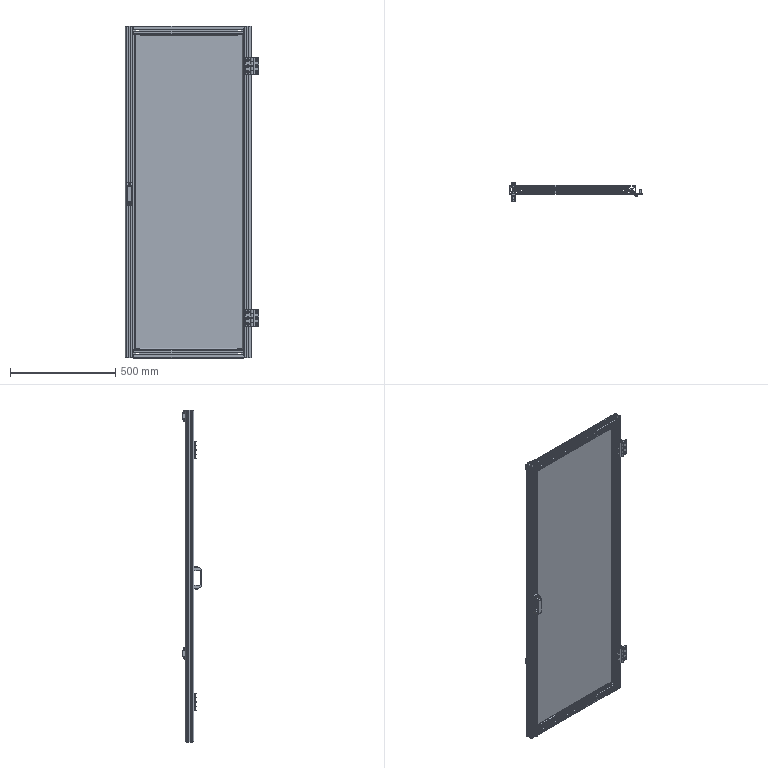Part | SolidWorks | features ReferencePattern 36, LocalLPattern 7, CompositeCurve 3 | 52 solids | 1971 faces | box 633 x 92.5 x 1575 mm | volume 6275343 mm3 | plane 1194 | cylinder 579 | cone 186 | spline 12 | commonest cylinder face diameters 2 x56 1.5 x48 20.854 x48 6.8 x40 6 x36 6.5 x28